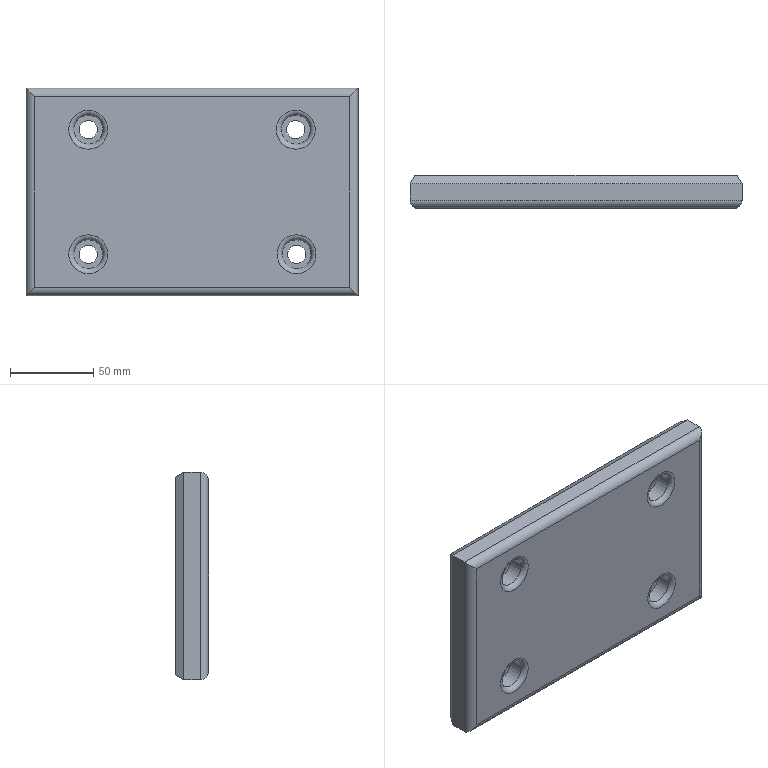Part | NX | features solid 2 | 1 solid | 30 faces | box 200 x 20 x 125 mm | volume 476702 mm3 | plane 14 | cylinder 12 | torus 4 | commonest cylinder face diameters 10 x4 11 x4 17.5 x4
STEP:
#1=CARTESIAN_POINT('',(-1142.5,-467.,221.25));
#2=VERTEX_POINT('',#1);
#3=CARTESIAN_POINT('',(-1142.5,-467.,230.));
#4=DIRECTION('',(0.,1.,0.));
#5=DIRECTION('',(0.,0.,-1.));
#6=AXIS2_PLACEMENT_3D('',#3,#4,#5);
#7=CIRCLE('',#6,8.75);
#8=EDGE_CURVE('',#2,#2,#7,.F.);
#9=ORIENTED_EDGE('',*,*,#8,.T.);
#10=EDGE_LOOP('',(#9));
#11=FACE_BOUND('',#10,.T.);
#12=CARTESIAN_POINT('',(-1142.5,-458.,221.25));
#13=VERTEX_POINT('',#12);
#14=CARTESIAN_POINT('',(-1142.5,-458.,230.));
#15=DIRECTION('',(0.,1.,0.));
#16=DIRECTION('',(0.,0.,-1.));
#17=AXIS2_PLACEMENT_3D('',#14,#15,#16);
#18=CIRCLE('',#17,8.75);
#19=EDGE_CURVE('',#13,#13,#18,.T.);
#20=ORIENTED_EDGE('',*,*,#19,.T.);
#21=EDGE_LOOP('',(#20));
#22=FACE_BOUND('',#21,.T.);
#23=CARTESIAN_POINT('',(-1142.5,-470.,230.));
#24=DIRECTION('',(0.,1.,0.));
#25=DIRECTION('',(0.,0.,-1.));
#26=AXIS2_PLACEMENT_3D('',#23,#24,#25);
#27=CYLINDRICAL_SURFACE('',#26,8.75);
#28=ADVANCED_FACE('',(#11,#22),#27,.F.);
#29=CARTESIAN_POINT('',(-1142.5,-467.,146.25));
#30=VERTEX_POINT('',#29);
#31=CARTESIAN_POINT('',(-1142.5,-467.,155.));
#32=DIRECTION('',(0.,1.,0.));
#33=DIRECTION('',(0.,0.,-1.));
#34=AXIS2_PLACEMENT_3D('',#31,#32,#33);
#35=CIRCLE('',#34,8.75);
#36=EDGE_CURVE('',#30,#30,#35,.F.);
#37=ORIENTED_EDGE('',*,*,#36,.T.);
#38=EDGE_LOOP('',(#37));
#39=FACE_BOUND('',#38,.T.);
#40=CARTESIAN_POINT('',(-1142.5,-458.,146.25));
#41=VERTEX_POINT('',#40);
#42=CARTESIAN_POINT('',(-1142.5,-458.,155.));
#43=DIRECTION('',(0.,1.,0.));
#44=DIRECTION('',(0.,0.,-1.));
#45=AXIS2_PLACEMENT_3D('',#42,#43,#44);
#46=CIRCLE('',#45,8.75);
#47=EDGE_CURVE('',#41,#41,#46,.T.);
#48=ORIENTED_EDGE('',*,*,#47,.T.);
#49=EDGE_LOOP('',(#48));
#50=FACE_BOUND('',#49,.T.);
#51=CARTESIAN_POINT('',(-1142.5,-470.,155.));
#52=DIRECTION('',(0.,1.,0.));
#53=DIRECTION('',(0.,0.,-1.));
#54=AXIS2_PLACEMENT_3D('',#51,#52,#53);
#55=CYLINDRICAL_SURFACE('',#54,8.75);
#56=ADVANCED_FACE('',(#39,#50),#55,.F.);
#57=CARTESIAN_POINT('',(-1142.5,-458.,224.5));
#58=VERTEX_POINT('',#57);
#59=CARTESIAN_POINT('',(-1142.5,-458.,230.));
#60=DIRECTION('',(0.,1.,0.));
#61=DIRECTION('',(0.,0.,-1.));
#62=AXIS2_PLACEMENT_3D('',#59,#60,#61);
#63=CIRCLE('',#62,5.5);
#64=EDGE_CURVE('',#58,#58,#63,.T.);
#65=ORIENTED_EDGE('',*,*,#64,.T.);
#66=EDGE_LOOP('',(#65));
#67=FACE_BOUND('',#66,.T.);
#68=ORIENTED_EDGE('',*,*,#19,.F.);
#69=EDGE_LOOP('',(#68));
#70=FACE_BOUND('',#69,.T.);
#71=CARTESIAN_POINT('',(-1142.5,-458.,230.));
#72=DIRECTION('',(0.,1.,0.));
#73=DIRECTION('',(0.,0.,-1.));
#74=AXIS2_PLACEMENT_3D('',#71,#72,#73);
#75=PLANE('',#74);
#76=ADVANCED_FACE('',(#67,#70),#75,.F.);
#77=CARTESIAN_POINT('',(-1142.5,-458.,149.5));
#78=VERTEX_POINT('',#77);
#79=CARTESIAN_POINT('',(-1142.5,-458.,155.));
#80=DIRECTION('',(0.,1.,0.));
#81=DIRECTION('',(0.,0.,-1.));
#82=AXIS2_PLACEMENT_3D('',#79,#80,#81);
#83=CIRCLE('',#82,5.5);
#84=EDGE_CURVE('',#78,#78,#83,.T.);
#85=ORIENTED_EDGE('',*,*,#84,.T.);
#86=EDGE_LOOP('',(#85));
#87=FACE_BOUND('',#86,.T.);
#88=ORIENTED_EDGE('',*,*,#47,.F.);
#89=EDGE_LOOP('',(#88));
#90=FACE_BOUND('',#89,.T.);
#91=CARTESIAN_POINT('',(-1142.5,-458.,155.));
#92=DIRECTION('',(0.,1.,0.));
#93=DIRECTION('',(0.,0.,-1.));
#94=AXIS2_PLACEMENT_3D('',#91,#92,#93);
#95=PLANE('',#94);
#96=ADVANCED_FACE('',(#87,#90),#95,.F.);
#97=CARTESIAN_POINT('',(-1180.,-465.,255.));
#98=VERTEX_POINT('',#97);
#99=CARTESIAN_POINT('',(-1180.,-455.,255.));
#100=VERTEX_POINT('',#99);
#101=CARTESIAN_POINT('',(-1180.,-470.,255.));
#102=DIRECTION('',(0.,1.,0.));
#103=VECTOR('',#102,1000.);
#104=LINE('',#101,#103);
#105=EDGE_CURVE('',#98,#100,#104,.T.);
#106=ORIENTED_EDGE('',*,*,#105,.T.);
#107=CARTESIAN_POINT('',(-1180.,-455.,130.));
#108=VERTEX_POINT('',#107);
#109=CARTESIAN_POINT('',(-1180.,-455.,200.));
#110=DIRECTION('',(0.,0.,-1.));
#111=VECTOR('',#110,1000.);
#112=LINE('',#109,#111);
#113=EDGE_CURVE('',#100,#108,#112,.T.);
#114=ORIENTED_EDGE('',*,*,#113,.T.);
#115=CARTESIAN_POINT('',(-1180.,-465.,130.));
#116=VERTEX_POINT('',#115);
#117=CARTESIAN_POINT('',(-1180.,-470.,130.));
#118=DIRECTION('',(0.,1.,0.));
#119=VECTOR('',#118,1000.);
#120=LINE('',#117,#119);
#121=EDGE_CURVE('',#116,#108,#120,.T.);
#122=ORIENTED_EDGE('',*,*,#121,.F.);
#123=CARTESIAN_POINT('',(-1180.,-465.,255.));
#124=DIRECTION('',(0.,0.,1.));
#125=VECTOR('',#124,1000.);
#126=LINE('',#123,#125);
#127=EDGE_CURVE('',#116,#98,#126,.T.);
#128=ORIENTED_EDGE('',*,*,#127,.T.);
#129=EDGE_LOOP('',(#106,#114,#122,#128));
#130=FACE_BOUND('',#129,.T.);
#131=CARTESIAN_POINT('',(-1180.,-470.,200.));
#132=DIRECTION('',(1.,0.,0.));
#133=DIRECTION('',(0.,0.,-1.));
#134=AXIS2_PLACEMENT_3D('',#131,#132,#133);
#135=PLANE('',#134);
#136=ADVANCED_FACE('',(#130),#135,.F.);
#137=ORIENTED_EDGE('',*,*,#8,.F.);
#138=EDGE_LOOP('',(#137));
#139=FACE_BOUND('',#138,.T.);
#140=CARTESIAN_POINT('',(-1142.5,-470.,218.25));
#141=VERTEX_POINT('',#140);
#142=CARTESIAN_POINT('',(-1142.5,-470.,230.));
#143=DIRECTION('',(0.,1.,0.));
#144=DIRECTION('',(0.,0.,-1.));
#145=AXIS2_PLACEMENT_3D('',#142,#143,#144);
#146=CIRCLE('',#145,11.75);
#147=EDGE_CURVE('',#141,#141,#146,.T.);
#148=ORIENTED_EDGE('',*,*,#147,.F.);
#149=EDGE_LOOP('',(#148));
#150=FACE_BOUND('',#149,.T.);
#151=CARTESIAN_POINT('',(-1142.5,-467.,230.));
#152=DIRECTION('',(0.,1.,0.));
#153=DIRECTION('',(0.,0.,-1.));
#154=AXIS2_PLACEMENT_3D('',#151,#152,#153);
#155=TOROIDAL_SURFACE('',#154,11.75,3.);
#156=ADVANCED_FACE('',(#139,#150),#155,.T.);
#157=ORIENTED_EDGE('',*,*,#36,.F.);
#158=EDGE_LOOP('',(#157));
#159=FACE_BOUND('',#158,.T.);
#160=CARTESIAN_POINT('',(-1142.5,-470.,143.25));
#161=VERTEX_POINT('',#160);
#162=CARTESIAN_POINT('',(-1142.5,-470.,155.));
#163=DIRECTION('',(0.,1.,0.));
#164=DIRECTION('',(0.,0.,-1.));
#165=AXIS2_PLACEMENT_3D('',#162,#163,#164);
#166=CIRCLE('',#165,11.75);
#167=EDGE_CURVE('',#161,#161,#166,.T.);
#168=ORIENTED_EDGE('',*,*,#167,.F.);
#169=EDGE_LOOP('',(#168));
#170=FACE_BOUND('',#169,.T.);
#171=CARTESIAN_POINT('',(-1142.5,-467.,155.));
#172=DIRECTION('',(0.,1.,0.));
#173=DIRECTION('',(0.,0.,-1.));
#174=AXIS2_PLACEMENT_3D('',#171,#172,#173);
#175=TOROIDAL_SURFACE('',#174,11.75,3.);
#176=ADVANCED_FACE('',(#159,#170),#175,.T.);
#177=ORIENTED_EDGE('',*,*,#64,.F.);
#178=EDGE_LOOP('',(#177));
#179=FACE_BOUND('',#178,.T.);
#180=CARTESIAN_POINT('',(-1142.5,-450.,224.5));
#181=VERTEX_POINT('',#180);
#182=CARTESIAN_POINT('',(-1142.5,-450.,230.));
#183=DIRECTION('',(0.,1.,0.));
#184=DIRECTION('',(0.,0.,-1.));
#185=AXIS2_PLACEMENT_3D('',#182,#183,#184);
#186=CIRCLE('',#185,5.5);
#187=EDGE_CURVE('',#181,#181,#186,.F.);
#188=ORIENTED_EDGE('',*,*,#187,.F.);
#189=EDGE_LOOP('',(#188));
#190=FACE_BOUND('',#189,.T.);
#191=CARTESIAN_POINT('',(-1142.5,-420.,230.));
#192=DIRECTION('',(0.,1.,0.));
#193=DIRECTION('',(0.,0.,-1.));
#194=AXIS2_PLACEMENT_3D('',#191,#192,#193);
#195=CYLINDRICAL_SURFACE('',#194,5.5);
#196=ADVANCED_FACE('',(#179,#190),#195,.F.);
#197=ORIENTED_EDGE('',*,*,#84,.F.);
#198=EDGE_LOOP('',(#197));
#199=FACE_BOUND('',#198,.T.);
#200=CARTESIAN_POINT('',(-1142.5,-450.,149.5));
#201=VERTEX_POINT('',#200);
#202=CARTESIAN_POINT('',(-1142.5,-450.,155.));
#203=DIRECTION('',(0.,1.,0.));
#204=DIRECTION('',(0.,0.,-1.));
#205=AXIS2_PLACEMENT_3D('',#202,#203,#204);
#206=CIRCLE('',#205,5.5);
#207=EDGE_CURVE('',#201,#201,#206,.F.);
#208=ORIENTED_EDGE('',*,*,#207,.F.);
#209=EDGE_LOOP('',(#208));
#210=FACE_BOUND('',#209,.T.);
#211=CARTESIAN_POINT('',(-1142.5,-420.,155.));
#212=DIRECTION('',(0.,1.,0.));
#213=DIRECTION('',(0.,0.,-1.));
#214=AXIS2_PLACEMENT_3D('',#211,#212,#213);
#215=CYLINDRICAL_SURFACE('',#214,5.5);
#216=ADVANCED_FACE('',(#199,#210),#215,.F.);
#217=CARTESIAN_POINT('',(-1175.,-470.,135.));
#218=VERTEX_POINT('',#217);
#219=CARTESIAN_POINT('',(-1175.,-465.,135.));
#220=DIRECTION('',(0.7071,0.,-0.7071));
#221=DIRECTION('',(0.7071,0.,0.7071));
#222=AXIS2_PLACEMENT_3D('',#219,#220,#221);
#223=ELLIPSE('',#222,7.071,5.);
#224=EDGE_CURVE('',#116,#218,#223,.F.);
#225=ORIENTED_EDGE('',*,*,#224,.T.);
#226=CARTESIAN_POINT('',(-1175.,-470.,250.));
#227=VERTEX_POINT('',#226);
#228=CARTESIAN_POINT('',(-1175.,-470.,130.));
#229=DIRECTION('',(0.,0.,-1.));
#230=VECTOR('',#229,1000.);
#231=LINE('',#228,#230);
#232=EDGE_CURVE('',#227,#218,#231,.T.);
#233=ORIENTED_EDGE('',*,*,#232,.F.);
#234=CARTESIAN_POINT('',(-1175.,-465.,250.));
#235=DIRECTION('',(-0.7071,0.,-0.7071));
#236=DIRECTION('',(0.7071,0.,-0.7071));
#237=AXIS2_PLACEMENT_3D('',#234,#235,#236);
#238=ELLIPSE('',#237,7.071,5.);
#239=EDGE_CURVE('',#98,#227,#238,.F.);
#240=ORIENTED_EDGE('',*,*,#239,.F.);
#241=ORIENTED_EDGE('',*,*,#127,.F.);
#242=EDGE_LOOP('',(#225,#233,#240,#241));
#243=FACE_BOUND('',#242,.T.);
#244=CARTESIAN_POINT('',(-1175.,-465.,200.));
#245=DIRECTION('',(0.,0.,-1.));
#246=DIRECTION('',(0.,-1.,0.));
#247=AXIS2_PLACEMENT_3D('',#244,#245,#246);
#248=CYLINDRICAL_SURFACE('',#247,5.);
#249=ADVANCED_FACE('',(#243),#248,.T.);
#250=CARTESIAN_POINT('',(-1177.,-450.,252.));
#251=VERTEX_POINT('',#250);
#252=CARTESIAN_POINT('',(-1153.837,-411.395,228.837));
#253=DIRECTION('',(-0.4575,-0.7625,0.4575));
#254=VECTOR('',#253,1000.);
#255=LINE('',#252,#254);
#256=EDGE_CURVE('',#100,#251,#255,.F.);
#257=ORIENTED_EDGE('',*,*,#256,.T.);
#258=CARTESIAN_POINT('',(-1177.,-450.,133.));
#259=VERTEX_POINT('',#258);
#260=CARTESIAN_POINT('',(-1177.,-450.,200.));
#261=DIRECTION('',(0.,0.,-1.));
#262=VECTOR('',#261,1000.);
#263=LINE('',#260,#262);
#264=EDGE_CURVE('',#259,#251,#263,.F.);
#265=ORIENTED_EDGE('',*,*,#264,.F.);
#266=CARTESIAN_POINT('',(-1151.465,-407.442,158.535));
#267=DIRECTION('',(-0.4575,-0.7625,-0.4575));
#268=VECTOR('',#267,1000.);
#269=LINE('',#266,#268);
#270=EDGE_CURVE('',#259,#108,#269,.T.);
#271=ORIENTED_EDGE('',*,*,#270,.T.);
#272=ORIENTED_EDGE('',*,*,#113,.F.);
#273=EDGE_LOOP('',(#257,#265,#271,#272));
#274=FACE_BOUND('',#273,.T.);
#275=CARTESIAN_POINT('',(-1180.,-455.,200.));
#276=DIRECTION('',(-0.8575,0.5145,0.));
#277=DIRECTION('',(-0.5145,-0.8575,0.));
#278=AXIS2_PLACEMENT_3D('',#275,#276,#277);
#279=PLANE('',#278);
#280=ADVANCED_FACE('',(#274),#279,.T.);
#281=CARTESIAN_POINT('',(-985.,-470.,250.));
#282=VERTEX_POINT('',#281);
#283=CARTESIAN_POINT('',(-1180.,-470.,250.));
#284=DIRECTION('',(-1.,0.,0.));
#285=VECTOR('',#284,1000.);
#286=LINE('',#283,#285);
#287=EDGE_CURVE('',#282,#227,#286,.T.);
#288=ORIENTED_EDGE('',*,*,#287,.F.);
#289=CARTESIAN_POINT('',(-980.,-465.,255.));
#290=VERTEX_POINT('',#289);
#291=CARTESIAN_POINT('',(-985.,-465.,250.));
#292=DIRECTION('',(-0.7071,0.,0.7071));
#293=DIRECTION('',(0.7071,0.,0.7071));
#294=AXIS2_PLACEMENT_3D('',#291,#292,#293);
#295=ELLIPSE('',#294,7.071,5.);
#296=EDGE_CURVE('',#282,#290,#295,.T.);
#297=ORIENTED_EDGE('',*,*,#296,.T.);
#298=CARTESIAN_POINT('',(-1055.,-465.,255.));
#299=DIRECTION('',(1.,0.,0.));
#300=VECTOR('',#299,1000.);
#301=LINE('',#298,#300);
#302=EDGE_CURVE('',#98,#290,#301,.T.);
#303=ORIENTED_EDGE('',*,*,#302,.F.);
#304=ORIENTED_EDGE('',*,*,#239,.T.);
#305=EDGE_LOOP('',(#288,#297,#303,#304));
#306=FACE_BOUND('',#305,.T.);
#307=CARTESIAN_POINT('',(-1055.,-465.,250.));
#308=DIRECTION('',(-1.,0.,0.));
#309=DIRECTION('',(0.,0.,1.));
#310=AXIS2_PLACEMENT_3D('',#307,#308,#309);
#311=CYLINDRICAL_SURFACE('',#310,5.);
#312=ADVANCED_FACE('',(#306),#311,.T.);
#313=CARTESIAN_POINT('',(-980.,-465.,130.));
#314=VERTEX_POINT('',#313);
#315=CARTESIAN_POINT('',(-1055.,-465.,130.));
#316=DIRECTION('',(1.,0.,0.));
#317=VECTOR('',#316,1000.);
#318=LINE('',#315,#317);
#319=EDGE_CURVE('',#314,#116,#318,.F.);
#320=ORIENTED_EDGE('',*,*,#319,.F.);
#321=CARTESIAN_POINT('',(-985.,-470.,135.));
#322=VERTEX_POINT('',#321);
#323=CARTESIAN_POINT('',(-985.,-465.,135.));
#324=DIRECTION('',(0.7071,0.,0.7071));
#325=DIRECTION('',(-0.7071,0.,0.7071));
#326=AXIS2_PLACEMENT_3D('',#323,#324,#325);
#327=ELLIPSE('',#326,7.071,5.);
#328=EDGE_CURVE('',#322,#314,#327,.T.);
#329=ORIENTED_EDGE('',*,*,#328,.F.);
#330=CARTESIAN_POINT('',(-1055.,-470.,135.));
#331=DIRECTION('',(-1.,0.,0.));
#332=VECTOR('',#331,1000.);
#333=LINE('',#330,#332);
#334=EDGE_CURVE('',#218,#322,#333,.F.);
#335=ORIENTED_EDGE('',*,*,#334,.F.);
#336=ORIENTED_EDGE('',*,*,#224,.F.);
#337=EDGE_LOOP('',(#320,#329,#335,#336));
#338=FACE_BOUND('',#337,.T.);
#339=CARTESIAN_POINT('',(-1055.,-465.,135.));
#340=DIRECTION('',(1.,0.,0.));
#341=DIRECTION('',(0.,0.,-1.));
#342=AXIS2_PLACEMENT_3D('',#339,#340,#341);
#343=CYLINDRICAL_SURFACE('',#342,5.);
#344=ADVANCED_FACE('',(#338),#343,.T.);
#345=ORIENTED_EDGE('',*,*,#167,.T.);
#346=EDGE_LOOP('',(#345));
#347=FACE_BOUND('',#346,.T.);
#348=ORIENTED_EDGE('',*,*,#147,.T.);
#349=EDGE_LOOP('',(#348));
#350=FACE_BOUND('',#349,.T.);
#351=ORIENTED_EDGE('',*,*,#334,.T.);
#352=CARTESIAN_POINT('',(-985.,-470.,200.));
#353=DIRECTION('',(0.,0.,-1.));
#354=VECTOR('',#353,1000.);
#355=LINE('',#352,#354);
#356=EDGE_CURVE('',#322,#282,#355,.F.);
#357=ORIENTED_EDGE('',*,*,#356,.T.);
#358=ORIENTED_EDGE('',*,*,#287,.T.);
#359=ORIENTED_EDGE('',*,*,#232,.T.);
#360=EDGE_LOOP('',(#351,#357,#358,#359));
#361=FACE_BOUND('',#360,.T.);
#362=CARTESIAN_POINT('',(-1017.5,-470.,218.25));
#363=VERTEX_POINT('',#362);
#364=CARTESIAN_POINT('',(-1017.5,-470.,230.));
#365=DIRECTION('',(0.,1.,0.));
#366=DIRECTION('',(0.,0.,-1.));
#367=AXIS2_PLACEMENT_3D('',#364,#365,#366);
#368=CIRCLE('',#367,11.75);
#369=EDGE_CURVE('',#363,#363,#368,.T.);
#370=ORIENTED_EDGE('',*,*,#369,.T.);
#371=EDGE_LOOP('',(#370));
#372=FACE_BOUND('',#371,.T.);
#373=CARTESIAN_POINT('',(-1017.,-470.,143.25));
#374=VERTEX_POINT('',#373);
#375=CARTESIAN_POINT('',(-1017.,-470.,155.));
#376=DIRECTION('',(0.,1.,0.));
#377=DIRECTION('',(0.,0.,-1.));
#378=AXIS2_PLACEMENT_3D('',#375,#376,#377);
#379=CIRCLE('',#378,11.75);
#380=EDGE_CURVE('',#374,#374,#379,.T.);
#381=ORIENTED_EDGE('',*,*,#380,.T.);
#382=EDGE_LOOP('',(#381));
#383=FACE_BOUND('',#382,.T.);
#384=CARTESIAN_POINT('',(-1055.,-470.,200.));
#385=DIRECTION('',(0.,1.,0.));
#386=DIRECTION('',(0.,0.,-1.));
#387=AXIS2_PLACEMENT_3D('',#384,#385,#386);
#388=PLANE('',#387);
#389=ADVANCED_FACE('',(#347,#350,#361,#372,#383),#388,.F.);
#390=CARTESIAN_POINT('',(-980.,-455.,255.));
#391=VERTEX_POINT('',#390);
#392=CARTESIAN_POINT('',(-1055.,-455.,255.));
#393=DIRECTION('',(-1.,0.,0.));
#394=VECTOR('',#393,1000.);
#395=LINE('',#392,#394);
#396=EDGE_CURVE('',#391,#100,#395,.T.);
#397=ORIENTED_EDGE('',*,*,#396,.F.);
#398=CARTESIAN_POINT('',(-983.,-450.,252.));
#399=VERTEX_POINT('',#398);
#400=CARTESIAN_POINT('',(-993.884,-431.86,241.116));
#401=DIRECTION('',(-0.4575,0.7625,-0.4575));
#402=VECTOR('',#401,1000.);
#403=LINE('',#400,#402);
#404=EDGE_CURVE('',#391,#399,#403,.T.);
#405=ORIENTED_EDGE('',*,*,#404,.T.);
#406=CARTESIAN_POINT('',(-1055.,-450.,252.));
#407=DIRECTION('',(-1.,0.,0.));
#408=VECTOR('',#407,1000.);
#409=LINE('',#406,#408);
#410=EDGE_CURVE('',#251,#399,#409,.F.);
#411=ORIENTED_EDGE('',*,*,#410,.F.);
#412=ORIENTED_EDGE('',*,*,#256,.F.);
#413=EDGE_LOOP('',(#397,#405,#411,#412));
#414=FACE_BOUND('',#413,.T.);
#415=CARTESIAN_POINT('',(-1055.,-455.,255.));
#416=DIRECTION('',(0.,0.5145,0.8575));
#417=DIRECTION('',(0.,0.8575,-0.5145));
#418=AXIS2_PLACEMENT_3D('',#415,#416,#417);
#419=PLANE('',#418);
#420=ADVANCED_FACE('',(#414),#419,.T.);
#421=CARTESIAN_POINT('',(-983.,-450.,133.));
#422=VERTEX_POINT('',#421);
#423=CARTESIAN_POINT('',(-1180.,-450.,133.));
#424=DIRECTION('',(1.,0.,0.));
#425=VECTOR('',#424,1000.);
#426=LINE('',#423,#425);
#427=EDGE_CURVE('',#422,#259,#426,.F.);
#428=ORIENTED_EDGE('',*,*,#427,.F.);
#429=CARTESIAN_POINT('',(-980.,-455.,130.));
#430=VERTEX_POINT('',#429);
#431=CARTESIAN_POINT('',(-997.023,-426.628,147.023));
#432=DIRECTION('',(-0.4575,0.7625,0.4575));
#433=VECTOR('',#432,1000.);
#434=LINE('',#431,#433);
#435=EDGE_CURVE('',#422,#430,#434,.F.);
#436=ORIENTED_EDGE('',*,*,#435,.T.);
#437=CARTESIAN_POINT('',(-1055.,-455.,130.));
#438=DIRECTION('',(1.,0.,0.));
#439=VECTOR('',#438,1000.);
#440=LINE('',#437,#439);
#441=EDGE_CURVE('',#108,#430,#440,.T.);
#442=ORIENTED_EDGE('',*,*,#441,.F.);
#443=ORIENTED_EDGE('',*,*,#270,.F.);
#444=EDGE_LOOP('',(#428,#436,#442,#443));
#445=FACE_BOUND('',#444,.T.);
#446=CARTESIAN_POINT('',(-1055.,-450.,133.));
#447=DIRECTION('',(0.,-0.5145,0.8575));
#448=DIRECTION('',(0.,0.8575,0.5145));
#449=AXIS2_PLACEMENT_3D('',#446,#447,#448);
#450=PLANE('',#449);
#451=ADVANCED_FACE('',(#445),#450,.F.);
#452=ORIENTED_EDGE('',*,*,#207,.T.);
#453=EDGE_LOOP('',(#452));
#454=FACE_BOUND('',#453,.T.);
#455=ORIENTED_EDGE('',*,*,#187,.T.);
#456=EDGE_LOOP('',(#455));
#457=FACE_BOUND('',#456,.T.);
#458=ORIENTED_EDGE('',*,*,#410,.T.);
#459=CARTESIAN_POINT('',(-983.,-450.,130.));
#460=DIRECTION('',(0.,0.,1.));
#461=VECTOR('',#460,1000.);
#462=LINE('',#459,#461);
#463=EDGE_CURVE('',#399,#422,#462,.F.);
#464=ORIENTED_EDGE('',*,*,#463,.T.);
#465=ORIENTED_EDGE('',*,*,#427,.T.);
#466=ORIENTED_EDGE('',*,*,#264,.T.);
#467=EDGE_LOOP('',(#458,#464,#465,#466));
#468=FACE_BOUND('',#467,.T.);
#469=CARTESIAN_POINT('',(-1017.5,-450.,224.5));
#470=VERTEX_POINT('',#469);
#471=CARTESIAN_POINT('',(-1017.5,-450.,230.));
#472=DIRECTION('',(0.,1.,0.));
#473=DIRECTION('',(0.,0.,-1.));
#474=AXIS2_PLACEMENT_3D('',#471,#472,#473);
#475=CIRCLE('',#474,5.5);
#476=EDGE_CURVE('',#470,#470,#475,.F.);
#477=ORIENTED_EDGE('',*,*,#476,.T.);
#478=EDGE_LOOP('',(#477));
#479=FACE_BOUND('',#478,.T.);
#480=CARTESIAN_POINT('',(-1017.,-450.,149.5));
#481=VERTEX_POINT('',#480);
#482=CARTESIAN_POINT('',(-1017.,-450.,155.));
#483=DIRECTION('',(0.,1.,0.));
#484=DIRECTION('',(0.,0.,-1.));
#485=AXIS2_PLACEMENT_3D('',#482,#483,#484);
#486=CIRCLE('',#485,5.5);
#487=EDGE_CURVE('',#481,#481,#486,.F.);
#488=ORIENTED_EDGE('',*,*,#487,.T.);
#489=EDGE_LOOP('',(#488));
#490=FACE_BOUND('',#489,.T.);
#491=CARTESIAN_POINT('',(-1055.,-450.,200.));
#492=DIRECTION('',(0.,1.,0.));
#493=DIRECTION('',(0.,0.,-1.));
#494=AXIS2_PLACEMENT_3D('',#491,#492,#493);
#495=PLANE('',#494);
#496=ADVANCED_FACE('',(#454,#457,#468,#479,#490),#495,.T.);
#497=ORIENTED_EDGE('',*,*,#302,.T.);
#498=CARTESIAN_POINT('',(-980.,-470.,255.));
#499=DIRECTION('',(0.,1.,0.));
#500=VECTOR('',#499,1000.);
#501=LINE('',#498,#500);
#502=EDGE_CURVE('',#290,#391,#501,.T.);
#503=ORIENTED_EDGE('',*,*,#502,.T.);
#504=ORIENTED_EDGE('',*,*,#396,.T.);
#505=ORIENTED_EDGE('',*,*,#105,.F.);
#506=EDGE_LOOP('',(#497,#503,#504,#505));
#507=FACE_BOUND('',#506,.T.);
#508=CARTESIAN_POINT('',(-1055.,-470.,255.));
#509=DIRECTION('',(0.,0.,-1.));
#510=DIRECTION('',(0.,-1.,0.));
#511=AXIS2_PLACEMENT_3D('',#508,#509,#510);
#512=PLANE('',#511);
#513=ADVANCED_FACE('',(#507),#512,.F.);
#514=ORIENTED_EDGE('',*,*,#441,.T.);
#515=CARTESIAN_POINT('',(-980.,-455.,130.));
#516=CARTESIAN_POINT('',(-980.,-458.333,130.));
#517=CARTESIAN_POINT('',(-980.,-461.667,130.));
#518=CARTESIAN_POINT('',(-980.,-465.,130.));
#519=B_SPLINE_CURVE_WITH_KNOTS('',3,(#515,#516,#517,#518),.UNSPECIFIED.,.F.,.F.,(4,4),(0.25,0.75),.UNSPECIFIED.);
#520=EDGE_CURVE('',#314,#430,#519,.F.);
#521=ORIENTED_EDGE('',*,*,#520,.F.);
#522=ORIENTED_EDGE('',*,*,#319,.T.);
#523=ORIENTED_EDGE('',*,*,#121,.T.);
#524=EDGE_LOOP('',(#514,#521,#522,#523));
#525=FACE_BOUND('',#524,.T.);
#526=CARTESIAN_POINT('',(-1055.,-470.,130.));
#527=DIRECTION('',(0.,0.,-1.));
#528=DIRECTION('',(0.,-1.,0.));
#529=AXIS2_PLACEMENT_3D('',#526,#527,#528);
#530=PLANE('',#529);
#531=ADVANCED_FACE('',(#525),#530,.T.);
#532=ORIENTED_EDGE('',*,*,#520,.T.);
#533=CARTESIAN_POINT('',(-980.,-455.,255.));
#534=DIRECTION('',(0.,0.,1.));
#535=VECTOR('',#534,1000.);
#536=LINE('',#533,#535);
#537=EDGE_CURVE('',#430,#391,#536,.T.);
#538=ORIENTED_EDGE('',*,*,#537,.T.);
#539=ORIENTED_EDGE('',*,*,#502,.F.);
#540=CARTESIAN_POINT('',(-980.,-465.,200.));
#541=DIRECTION('',(0.,0.,1.));
#542=VECTOR('',#541,1000.);
#543=LINE('',#540,#542);
#544=EDGE_CURVE('',#290,#314,#543,.F.);
#545=ORIENTED_EDGE('',*,*,#544,.T.);
#546=EDGE_LOOP('',(#532,#538,#539,#545));
#547=FACE_BOUND('',#546,.T.);
#548=CARTESIAN_POINT('',(-980.,-470.,200.));
#549=DIRECTION('',(1.,0.,0.));
#550=DIRECTION('',(0.,0.,-1.));
#551=AXIS2_PLACEMENT_3D('',#548,#549,#550);
#552=PLANE('',#551);
#553=ADVANCED_FACE('',(#547),#552,.T.);
#554=CARTESIAN_POINT('',(-1017.,-458.,149.5));
#555=VERTEX_POINT('',#554);
#556=CARTESIAN_POINT('',(-1017.,-458.,155.));
#557=DIRECTION('',(0.,1.,0.));
#558=DIRECTION('',(0.,0.,-1.));
#559=AXIS2_PLACEMENT_3D('',#556,#557,#558);
#560=CIRCLE('',#559,5.5);
#561=EDGE_CURVE('',#555,#555,#560,.T.);
#562=ORIENTED_EDGE('',*,*,#561,.F.);
#563=EDGE_LOOP('',(#562));
#564=FACE_BOUND('',#563,.T.);
#565=ORIENTED_EDGE('',*,*,#487,.F.);
#566=EDGE_LOOP('',(#565));
#567=FACE_BOUND('',#566,.T.);
#568=CARTESIAN_POINT('',(-1017.,-420.,155.));
#569=DIRECTION('',(0.,1.,0.));
#570=DIRECTION('',(0.,0.,-1.));
#571=AXIS2_PLACEMENT_3D('',#568,#569,#570);
#572=CYLINDRICAL_SURFACE('',#571,5.5);
#573=ADVANCED_FACE('',(#564,#567),#572,.F.);
#574=ORIENTED_EDGE('',*,*,#561,.T.);
#575=EDGE_LOOP('',(#574));
#576=FACE_BOUND('',#575,.T.);
#577=CARTESIAN_POINT('',(-1017.,-458.,146.25));
#578=VERTEX_POINT('',#577);
#579=CARTESIAN_POINT('',(-1017.,-458.,155.));
#580=DIRECTION('',(0.,1.,0.));
#581=DIRECTION('',(0.,0.,-1.));
#582=AXIS2_PLACEMENT_3D('',#579,#580,#581);
#583=CIRCLE('',#582,8.75);
#584=EDGE_CURVE('',#578,#578,#583,.T.);
#585=ORIENTED_EDGE('',*,*,#584,.F.);
#586=EDGE_LOOP('',(#585));
#587=FACE_BOUND('',#586,.T.);
#588=CARTESIAN_POINT('',(-1017.,-458.,155.));
#589=DIRECTION('',(0.,1.,0.));
#590=DIRECTION('',(0.,0.,-1.));
#591=AXIS2_PLACEMENT_3D('',#588,#589,#590);
#592=PLANE('',#591);
#593=ADVANCED_FACE('',(#576,#587),#592,.F.);
#594=CARTESIAN_POINT('',(-1017.,-467.,146.25));
#595=VERTEX_POINT('',#594);
#596=CARTESIAN_POINT('',(-1017.,-467.,155.));
#597=DIRECTION('',(0.,1.,0.));
#598=DIRECTION('',(0.,0.,-1.));
#599=AXIS2_PLACEMENT_3D('',#596,#597,#598);
#600=CIRCLE('',#599,8.75);
#601=EDGE_CURVE('',#595,#595,#600,.F.);
#602=ORIENTED_EDGE('',*,*,#601,.T.);
#603=EDGE_LOOP('',(#602));
#604=FACE_BOUND('',#603,.T.);
#605=ORIENTED_EDGE('',*,*,#584,.T.);
#606=EDGE_LOOP('',(#605));
#607=FACE_BOUND('',#606,.T.);
#608=CARTESIAN_POINT('',(-1017.,-470.,155.));
#609=DIRECTION('',(0.,1.,0.));
#610=DIRECTION('',(0.,0.,-1.));
#611=AXIS2_PLACEMENT_3D('',#608,#609,#610);
#612=CYLINDRICAL_SURFACE('',#611,8.75);
#613=ADVANCED_FACE('',(#604,#607),#612,.F.);
#614=CARTESIAN_POINT('',(-1017.5,-458.,224.5));
#615=VERTEX_POINT('',#614);
#616=CARTESIAN_POINT('',(-1017.5,-458.,230.));
#617=DIRECTION('',(0.,1.,0.));
#618=DIRECTION('',(0.,0.,-1.));
#619=AXIS2_PLACEMENT_3D('',#616,#617,#618);
#620=CIRCLE('',#619,5.5);
#621=EDGE_CURVE('',#615,#615,#620,.T.);
#622=ORIENTED_EDGE('',*,*,#621,.F.);
#623=EDGE_LOOP('',(#622));
#624=FACE_BOUND('',#623,.T.);
#625=ORIENTED_EDGE('',*,*,#476,.F.);
#626=EDGE_LOOP('',(#625));
#627=FACE_BOUND('',#626,.T.);
#628=CARTESIAN_POINT('',(-1017.5,-420.,230.));
#629=DIRECTION('',(0.,1.,0.));
#630=DIRECTION('',(0.,0.,-1.));
#631=AXIS2_PLACEMENT_3D('',#628,#629,#630);
#632=CYLINDRICAL_SURFACE('',#631,5.5);
#633=ADVANCED_FACE('',(#624,#627),#632,.F.);
#634=ORIENTED_EDGE('',*,*,#621,.T.);
#635=EDGE_LOOP('',(#634));
#636=FACE_BOUND('',#635,.T.);
#637=CARTESIAN_POINT('',(-1017.5,-458.,221.25));
#638=VERTEX_POINT('',#637);
#639=CARTESIAN_POINT('',(-1017.5,-458.,230.));
#640=DIRECTION('',(0.,1.,0.));
#641=DIRECTION('',(0.,0.,-1.));
#642=AXIS2_PLACEMENT_3D('',#639,#640,#641);
#643=CIRCLE('',#642,8.75);
#644=EDGE_CURVE('',#638,#638,#643,.T.);
#645=ORIENTED_EDGE('',*,*,#644,.F.);
#646=EDGE_LOOP('',(#645));
#647=FACE_BOUND('',#646,.T.);
#648=CARTESIAN_POINT('',(-1017.5,-458.,230.));
#649=DIRECTION('',(0.,1.,0.));
#650=DIRECTION('',(0.,0.,-1.));
#651=AXIS2_PLACEMENT_3D('',#648,#649,#650);
#652=PLANE('',#651);
#653=ADVANCED_FACE('',(#636,#647),#652,.F.);
#654=CARTESIAN_POINT('',(-1017.5,-467.,221.25));
#655=VERTEX_POINT('',#654);
#656=CARTESIAN_POINT('',(-1017.5,-467.,230.));
#657=DIRECTION('',(0.,1.,0.));
#658=DIRECTION('',(0.,0.,-1.));
#659=AXIS2_PLACEMENT_3D('',#656,#657,#658);
#660=CIRCLE('',#659,8.75);
#661=EDGE_CURVE('',#655,#655,#660,.F.);
#662=ORIENTED_EDGE('',*,*,#661,.T.);
#663=EDGE_LOOP('',(#662));
#664=FACE_BOUND('',#663,.T.);
#665=ORIENTED_EDGE('',*,*,#644,.T.);
#666=EDGE_LOOP('',(#665));
#667=FACE_BOUND('',#666,.T.);
#668=CARTESIAN_POINT('',(-1017.5,-470.,230.));
#669=DIRECTION('',(0.,1.,0.));
#670=DIRECTION('',(0.,0.,-1.));
#671=AXIS2_PLACEMENT_3D('',#668,#669,#670);
#672=CYLINDRICAL_SURFACE('',#671,8.75);
#673=ADVANCED_FACE('',(#664,#667),#672,.F.);
#674=ORIENTED_EDGE('',*,*,#328,.T.);
#675=ORIENTED_EDGE('',*,*,#544,.F.);
#676=ORIENTED_EDGE('',*,*,#296,.F.);
#677=ORIENTED_EDGE('',*,*,#356,.F.);
#678=EDGE_LOOP('',(#674,#675,#676,#677));
#679=FACE_BOUND('',#678,.T.);
#680=CARTESIAN_POINT('',(-985.,-465.,200.));
#681=DIRECTION('',(0.,0.,1.));
#682=DIRECTION('',(0.,1.,0.));
#683=AXIS2_PLACEMENT_3D('',#680,#681,#682);
#684=CYLINDRICAL_SURFACE('',#683,5.);
#685=ADVANCED_FACE('',(#679),#684,.T.);
#686=ORIENTED_EDGE('',*,*,#661,.F.);
#687=EDGE_LOOP('',(#686));
#688=FACE_BOUND('',#687,.T.);
#689=ORIENTED_EDGE('',*,*,#369,.F.);
#690=EDGE_LOOP('',(#689));
#691=FACE_BOUND('',#690,.T.);
#692=CARTESIAN_POINT('',(-1017.5,-467.,230.));
#693=DIRECTION('',(0.,1.,0.));
#694=DIRECTION('',(0.,0.,-1.));
#695=AXIS2_PLACEMENT_3D('',#692,#693,#694);
#696=TOROIDAL_SURFACE('',#695,11.75,3.);
#697=ADVANCED_FACE('',(#688,#691),#696,.T.);
#698=ORIENTED_EDGE('',*,*,#601,.F.);
#699=EDGE_LOOP('',(#698));
#700=FACE_BOUND('',#699,.T.);
#701=ORIENTED_EDGE('',*,*,#380,.F.);
#702=EDGE_LOOP('',(#701));
#703=FACE_BOUND('',#702,.T.);
#704=CARTESIAN_POINT('',(-1017.,-467.,155.));
#705=DIRECTION('',(0.,1.,0.));
#706=DIRECTION('',(0.,0.,-1.));
#707=AXIS2_PLACEMENT_3D('',#704,#705,#706);
#708=TOROIDAL_SURFACE('',#707,11.75,3.);
#709=ADVANCED_FACE('',(#700,#703),#708,.T.);
#710=ORIENTED_EDGE('',*,*,#435,.F.);
#711=ORIENTED_EDGE('',*,*,#463,.F.);
#712=ORIENTED_EDGE('',*,*,#404,.F.);
#713=ORIENTED_EDGE('',*,*,#537,.F.);
#714=EDGE_LOOP('',(#710,#711,#712,#713));
#715=FACE_BOUND('',#714,.T.);
#716=CARTESIAN_POINT('',(-983.,-450.,200.));
#717=DIRECTION('',(-0.8575,-0.5145,0.));
#718=DIRECTION('',(0.5145,-0.8575,0.));
#719=AXIS2_PLACEMENT_3D('',#716,#717,#718);
#720=PLANE('',#719);
#721=ADVANCED_FACE('',(#715),#720,.F.);
#722=CLOSED_SHELL('',(#28,#56,#76,#96,#136,#156,#176,#196,#216,#249,#280,#312,#344,#389,#420,#451,#496,#513,#531,#553,#573,#593,#613,#633,#653,#673,#685,#697,#709,#721));
#723=MANIFOLD_SOLID_BREP('',#722);
#724=(LENGTH_UNIT()NAMED_UNIT(*)SI_UNIT(.MILLI.,.METRE.));
#725=UNCERTAINTY_MEASURE_WITH_UNIT(LENGTH_MEASURE(0.0508),#724,'','');
#726=(NAMED_UNIT(*)PLANE_ANGLE_UNIT()SI_UNIT($,.RADIAN.));
#727=(NAMED_UNIT(*)SI_UNIT($,.STERADIAN.)SOLID_ANGLE_UNIT());
#728=(GEOMETRIC_REPRESENTATION_CONTEXT(3)GLOBAL_UNCERTAINTY_ASSIGNED_CONTEXT((#725))GLOBAL_UNIT_ASSIGNED_CONTEXT((#724,#726,#727))REPRESENTATION_CONTEXT('',''));
#729=ADVANCED_BREP_SHAPE_REPRESENTATION('',(#723),#728);